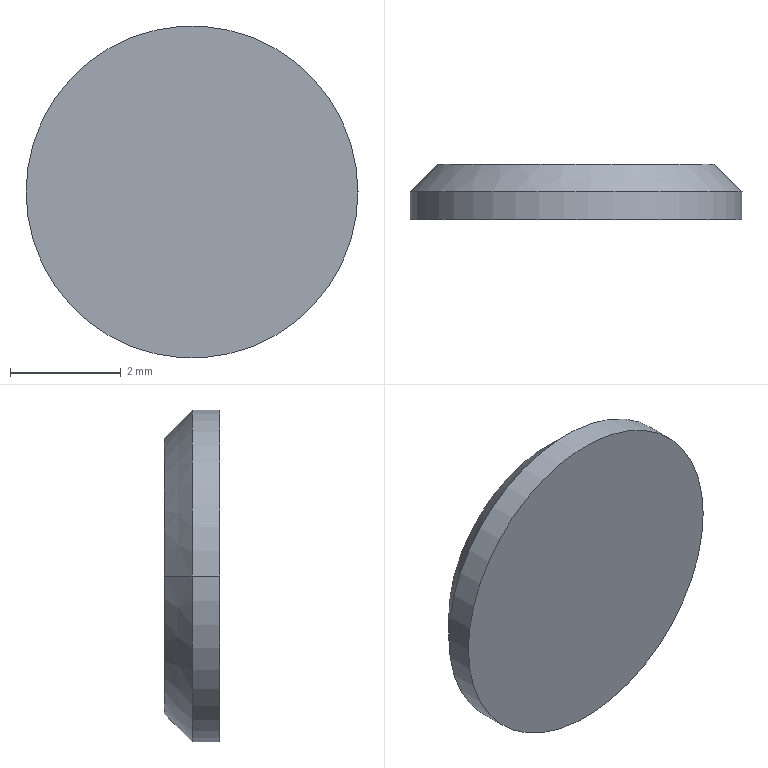Part | STEP file | 1 solid | 6 faces | box 6 x 1 x 6 mm | volume 26.049 mm3 | cylinder 2 | cone 2 | plane 2 | commonest cylinder face diameters 6 x2
STEP:
#1=CARTESIAN_POINT('',(3.,0.5,0.));
#2=VERTEX_POINT('',#1);
#3=CARTESIAN_POINT('',(-3.,0.5,0.));
#4=VERTEX_POINT('',#3);
#5=CARTESIAN_POINT('',(0.,0.5,0.));
#6=DIRECTION('',(0.,-1.,0.));
#7=DIRECTION('',(1.,0.,0.));
#8=AXIS2_PLACEMENT_3D('',#5,#6,#7);
#9=CIRCLE('',#8,3.);
#10=EDGE_CURVE('',#2,#4,#9,.T.);
#11=ORIENTED_EDGE('',*,*,#10,.T.);
#12=CARTESIAN_POINT('',(-3.,0.,0.));
#13=VERTEX_POINT('',#12);
#14=CARTESIAN_POINT('',(-3.,1.,0.));
#15=DIRECTION('',(0.,-1.,0.));
#16=VECTOR('',#15,1000.);
#17=LINE('',#14,#16);
#18=EDGE_CURVE('',#4,#13,#17,.T.);
#19=ORIENTED_EDGE('',*,*,#18,.T.);
#20=CARTESIAN_POINT('',(3.,0.,0.));
#21=VERTEX_POINT('',#20);
#22=CARTESIAN_POINT('',(0.,0.,0.));
#23=DIRECTION('',(0.,1.,0.));
#24=DIRECTION('',(1.,0.,0.));
#25=AXIS2_PLACEMENT_3D('',#22,#23,#24);
#26=CIRCLE('',#25,3.);
#27=EDGE_CURVE('',#13,#21,#26,.T.);
#28=ORIENTED_EDGE('',*,*,#27,.T.);
#29=CARTESIAN_POINT('',(3.,1.,0.));
#30=DIRECTION('',(0.,-1.,0.));
#31=VECTOR('',#30,1000.);
#32=LINE('',#29,#31);
#33=EDGE_CURVE('',#2,#21,#32,.T.);
#34=ORIENTED_EDGE('',*,*,#33,.F.);
#35=EDGE_LOOP('',(#11,#19,#28,#34));
#36=FACE_OUTER_BOUND('',#35,.T.);
#37=CARTESIAN_POINT('',(0.,1.,0.));
#38=DIRECTION('',(0.,-1.,0.));
#39=DIRECTION('',(1.,0.,0.));
#40=AXIS2_PLACEMENT_3D('',#37,#38,#39);
#41=CYLINDRICAL_SURFACE('',#40,3.);
#42=ADVANCED_FACE('',(#36),#41,.T.);
#43=CARTESIAN_POINT('',(2.5,1.,0.));
#44=VERTEX_POINT('',#43);
#45=CARTESIAN_POINT('',(-2.5,1.,0.));
#46=VERTEX_POINT('',#45);
#47=CARTESIAN_POINT('',(0.,1.,0.));
#48=DIRECTION('',(0.,-1.,0.));
#49=DIRECTION('',(1.,0.,0.));
#50=AXIS2_PLACEMENT_3D('',#47,#48,#49);
#51=CIRCLE('',#50,2.5);
#52=EDGE_CURVE('',#44,#46,#51,.T.);
#53=ORIENTED_EDGE('',*,*,#52,.T.);
#54=CARTESIAN_POINT('',(-3.,0.5,0.));
#55=DIRECTION('',(-0.7071,-0.7071,0.));
#56=VECTOR('',#55,1000.);
#57=LINE('',#54,#56);
#58=EDGE_CURVE('',#46,#4,#57,.T.);
#59=ORIENTED_EDGE('',*,*,#58,.T.);
#60=ORIENTED_EDGE('',*,*,#10,.F.);
#61=CARTESIAN_POINT('',(3.,0.5,0.));
#62=DIRECTION('',(0.7071,-0.7071,0.));
#63=VECTOR('',#62,1000.);
#64=LINE('',#61,#63);
#65=EDGE_CURVE('',#44,#2,#64,.T.);
#66=ORIENTED_EDGE('',*,*,#65,.F.);
#67=EDGE_LOOP('',(#53,#59,#60,#66));
#68=FACE_OUTER_BOUND('',#67,.T.);
#69=CARTESIAN_POINT('',(0.,0.5,0.));
#70=DIRECTION('',(0.,-1.,0.));
#71=DIRECTION('',(1.,0.,0.));
#72=AXIS2_PLACEMENT_3D('',#69,#70,#71);
#73=CONICAL_SURFACE('',#72,3.,0.7854);
#74=ADVANCED_FACE('',(#68),#73,.T.);
#75=CARTESIAN_POINT('',(0.,0.,0.));
#76=DIRECTION('',(0.,1.,0.));
#77=DIRECTION('',(1.,0.,0.));
#78=AXIS2_PLACEMENT_3D('',#75,#76,#77);
#79=CIRCLE('',#78,3.);
#80=EDGE_CURVE('',#21,#13,#79,.T.);
#81=ORIENTED_EDGE('',*,*,#80,.F.);
#82=ORIENTED_EDGE('',*,*,#27,.F.);
#83=EDGE_LOOP('',(#81,#82));
#84=FACE_OUTER_BOUND('',#83,.T.);
#85=CARTESIAN_POINT('',(0.,0.,0.));
#86=DIRECTION('',(0.,1.,0.));
#87=DIRECTION('',(1.,0.,0.));
#88=AXIS2_PLACEMENT_3D('',#85,#86,#87);
#89=PLANE('',#88);
#90=ADVANCED_FACE('',(#84),#89,.F.);
#91=ORIENTED_EDGE('',*,*,#18,.F.);
#92=CARTESIAN_POINT('',(0.,0.5,0.));
#93=DIRECTION('',(0.,-1.,0.));
#94=DIRECTION('',(1.,0.,0.));
#95=AXIS2_PLACEMENT_3D('',#92,#93,#94);
#96=CIRCLE('',#95,3.);
#97=EDGE_CURVE('',#4,#2,#96,.T.);
#98=ORIENTED_EDGE('',*,*,#97,.T.);
#99=ORIENTED_EDGE('',*,*,#33,.T.);
#100=ORIENTED_EDGE('',*,*,#80,.T.);
#101=EDGE_LOOP('',(#91,#98,#99,#100));
#102=FACE_OUTER_BOUND('',#101,.T.);
#103=CARTESIAN_POINT('',(0.,1.,0.));
#104=DIRECTION('',(0.,-1.,0.));
#105=DIRECTION('',(1.,0.,0.));
#106=AXIS2_PLACEMENT_3D('',#103,#104,#105);
#107=CYLINDRICAL_SURFACE('',#106,3.);
#108=ADVANCED_FACE('',(#102),#107,.T.);
#109=ORIENTED_EDGE('',*,*,#58,.F.);
#110=CARTESIAN_POINT('',(0.,1.,0.));
#111=DIRECTION('',(0.,-1.,0.));
#112=DIRECTION('',(1.,0.,0.));
#113=AXIS2_PLACEMENT_3D('',#110,#111,#112);
#114=CIRCLE('',#113,2.5);
#115=EDGE_CURVE('',#46,#44,#114,.T.);
#116=ORIENTED_EDGE('',*,*,#115,.T.);
#117=ORIENTED_EDGE('',*,*,#65,.T.);
#118=ORIENTED_EDGE('',*,*,#97,.F.);
#119=EDGE_LOOP('',(#109,#116,#117,#118));
#120=FACE_OUTER_BOUND('',#119,.T.);
#121=CARTESIAN_POINT('',(0.,0.5,0.));
#122=DIRECTION('',(0.,-1.,0.));
#123=DIRECTION('',(1.,0.,0.));
#124=AXIS2_PLACEMENT_3D('',#121,#122,#123);
#125=CONICAL_SURFACE('',#124,3.,0.7854);
#126=ADVANCED_FACE('',(#120),#125,.T.);
#127=ORIENTED_EDGE('',*,*,#52,.F.);
#128=ORIENTED_EDGE('',*,*,#115,.F.);
#129=EDGE_LOOP('',(#127,#128));
#130=FACE_OUTER_BOUND('',#129,.T.);
#131=CARTESIAN_POINT('',(0.,1.,0.));
#132=DIRECTION('',(0.,1.,0.));
#133=DIRECTION('',(1.,0.,0.));
#134=AXIS2_PLACEMENT_3D('',#131,#132,#133);
#135=PLANE('',#134);
#136=ADVANCED_FACE('',(#130),#135,.T.);
#137=CLOSED_SHELL('',(#42,#74,#90,#108,#126,#136));
#138=MANIFOLD_SOLID_BREP('',#137);
#139=CARTESIAN_POINT('',(0.,0.,0.));
#140=DIRECTION('',(0.,0.,1.));
#141=DIRECTION('',(1.,0.,0.));
#142=AXIS2_PLACEMENT_3D('',#139,#140,#141);
#143=(LENGTH_UNIT()NAMED_UNIT(*)SI_UNIT(.MILLI.,.METRE.));
#144=UNCERTAINTY_MEASURE_WITH_UNIT(LENGTH_MEASURE(0.00001),#143,'','');
#145=(NAMED_UNIT(*)PLANE_ANGLE_UNIT()SI_UNIT($,.RADIAN.));
#146=(NAMED_UNIT(*)SI_UNIT($,.STERADIAN.)SOLID_ANGLE_UNIT());
#147=(GEOMETRIC_REPRESENTATION_CONTEXT(3)GLOBAL_UNCERTAINTY_ASSIGNED_CONTEXT((#144))GLOBAL_UNIT_ASSIGNED_CONTEXT((#143,#145,#146))REPRESENTATION_CONTEXT('',''));
#148=ADVANCED_BREP_SHAPE_REPRESENTATION('',(#138,#142),#147);